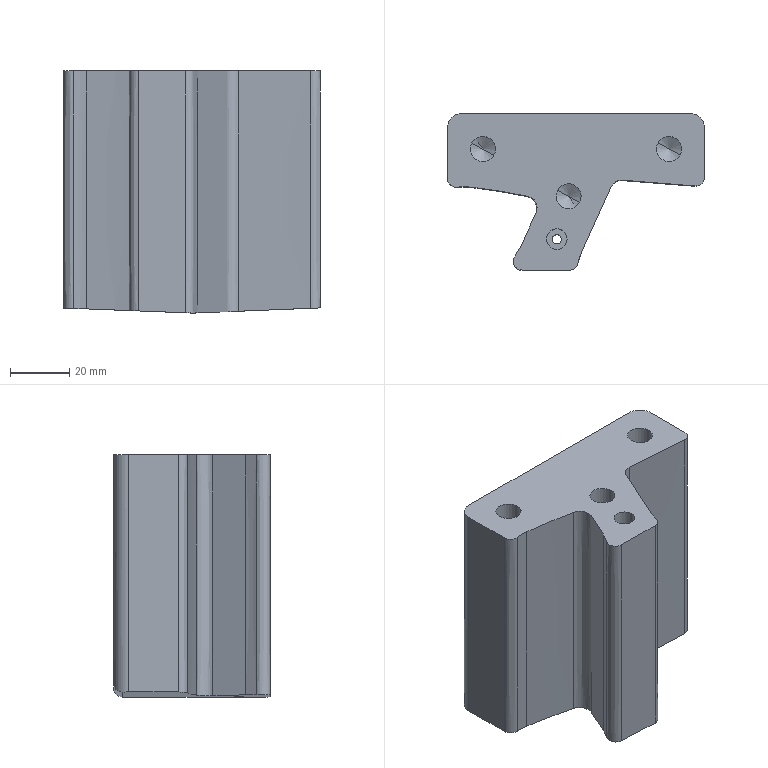Part | CATIA | 1 solid | 41 faces | box 87 x 53 x 82 mm | volume 218758 mm3 | cylinder 14 | other 12 | plane 9 | cone 6 | commonest cylinder face diameters 8.5 x6 3.2 x2 6 x2 7 x2 10 x2
STEP:
#1=CARTESIAN_POINT('',(-84.,32.5,41.546));
#2=VERTEX_POINT('',#1);
#3=CARTESIAN_POINT('',(-87.73,34.538,44.));
#4=VERTEX_POINT('',#3);
#5=CARTESIAN_POINT('',(-85.865,33.519,42.773));
#6=DIRECTION('',(-0.76,0.4152,0.5));
#7=VECTOR('',#6,1.);
#8=LINE('',#5,#7);
#9=EDGE_CURVE('',#2,#4,#8,.T.);
#10=ORIENTED_EDGE('',*,*,#9,.T.);
#11=CARTESIAN_POINT('',(-80.27,30.462,44.));
#12=VERTEX_POINT('',#11);
#13=CARTESIAN_POINT('',(-84.,32.5,44.));
#14=DIRECTION('',(0.,0.,1.));
#15=AXIS2_PLACEMENT_3D('',#13,#14,$);
#16=CIRCLE('',#15,4.25);
#17=EDGE_CURVE('',#12,#4,#16,.F.);
#18=ORIENTED_EDGE('',*,*,#17,.F.);
#19=CARTESIAN_POINT('',(-82.135,31.481,42.773));
#20=DIRECTION('',(0.76,-0.4152,0.5));
#21=VECTOR('',#20,1.);
#22=LINE('',#19,#21);
#23=EDGE_CURVE('',#2,#12,#22,.T.);
#24=ORIENTED_EDGE('',*,*,#23,.F.);
#25=EDGE_LOOP('',(#10,#18,#24));
#26=FACE_OUTER_BOUND('',#25,.T.);
#27=CARTESIAN_POINT('',(-84.,32.5,41.546));
#28=DIRECTION('',(0.,0.,1.));
#29=DIRECTION('',(0.8776,-0.4794,0.));
#30=AXIS2_PLACEMENT_3D('',#27,#28,#29);
#31=CONICAL_SURFACE('',#30,0.,1.047);
#32=ADVANCED_FACE('',(#26),#31,.F.);
#33=ORIENTED_EDGE('',*,*,#23,.T.);
#34=CARTESIAN_POINT('',(-84.,32.5,44.));
#35=DIRECTION('',(0.,0.,1.));
#36=AXIS2_PLACEMENT_3D('',#34,#35,$);
#37=CIRCLE('',#36,4.25);
#38=EDGE_CURVE('',#4,#12,#37,.F.);
#39=ORIENTED_EDGE('',*,*,#38,.F.);
#40=ORIENTED_EDGE('',*,*,#9,.F.);
#41=EDGE_LOOP('',(#33,#39,#40));
#42=FACE_OUTER_BOUND('',#41,.T.);
#43=ADVANCED_FACE('',(#42),#31,.F.);
#44=CARTESIAN_POINT('',(-87.73,34.538,69.));
#45=VERTEX_POINT('',#44);
#46=CARTESIAN_POINT('',(-80.27,30.462,69.));
#47=VERTEX_POINT('',#46);
#48=CARTESIAN_POINT('',(-84.,32.5,69.));
#49=DIRECTION('',(0.,0.,-1.));
#50=AXIS2_PLACEMENT_3D('',#48,#49,$);
#51=CIRCLE('',#50,4.25);
#52=EDGE_CURVE('',#45,#47,#51,.F.);
#53=ORIENTED_EDGE('',*,*,#52,.T.);
#54=CARTESIAN_POINT('',(-80.27,30.462,56.655));
#55=DIRECTION('',(0.,0.,-1.));
#56=VECTOR('',#55,1.);
#57=LINE('',#54,#56);
#58=EDGE_CURVE('',#12,#47,#57,.F.);
#59=ORIENTED_EDGE('',*,*,#58,.F.);
#60=ORIENTED_EDGE('',*,*,#17,.T.);
#61=CARTESIAN_POINT('',(-87.73,34.538,56.655));
#62=DIRECTION('',(0.,0.,-1.));
#63=VECTOR('',#62,1.);
#64=LINE('',#61,#63);
#65=EDGE_CURVE('',#4,#45,#64,.F.);
#66=ORIENTED_EDGE('',*,*,#65,.T.);
#67=EDGE_LOOP('',(#53,#59,#60,#66));
#68=FACE_OUTER_BOUND('',#67,.T.);
#69=CARTESIAN_POINT('',(-84.,32.5,68.9));
#70=DIRECTION('',(0.,0.,-1.));
#71=DIRECTION('',(0.8776,-0.4794,0.));
#72=AXIS2_PLACEMENT_3D('',#69,#70,#71);
#73=CYLINDRICAL_SURFACE('',#72,4.25);
#74=ADVANCED_FACE('',(#68),#73,.F.);
#75=CARTESIAN_POINT('',(-84.,32.5,69.));
#76=DIRECTION('',(0.,0.,-1.));
#77=AXIS2_PLACEMENT_3D('',#75,#76,$);
#78=CIRCLE('',#77,4.25);
#79=EDGE_CURVE('',#47,#45,#78,.F.);
#80=ORIENTED_EDGE('',*,*,#79,.T.);
#81=ORIENTED_EDGE('',*,*,#65,.F.);
#82=ORIENTED_EDGE('',*,*,#38,.T.);
#83=ORIENTED_EDGE('',*,*,#58,.T.);
#84=EDGE_LOOP('',(#80,#81,#82,#83));
#85=FACE_OUTER_BOUND('',#84,.T.);
#86=ADVANCED_FACE('',(#85),#73,.F.);
#87=CARTESIAN_POINT('',(-50.,48.5,41.546));
#88=VERTEX_POINT('',#87);
#89=CARTESIAN_POINT('',(-53.73,50.538,44.));
#90=VERTEX_POINT('',#89);
#91=CARTESIAN_POINT('',(-51.865,49.519,42.773));
#92=DIRECTION('',(-0.76,0.4152,0.5));
#93=VECTOR('',#92,1.);
#94=LINE('',#91,#93);
#95=EDGE_CURVE('',#88,#90,#94,.T.);
#96=ORIENTED_EDGE('',*,*,#95,.T.);
#97=CARTESIAN_POINT('',(-46.27,46.462,44.));
#98=VERTEX_POINT('',#97);
#99=CARTESIAN_POINT('',(-50.,48.5,44.));
#100=DIRECTION('',(0.,0.,1.));
#101=AXIS2_PLACEMENT_3D('',#99,#100,$);
#102=CIRCLE('',#101,4.25);
#103=EDGE_CURVE('',#98,#90,#102,.F.);
#104=ORIENTED_EDGE('',*,*,#103,.F.);
#105=CARTESIAN_POINT('',(-48.135,47.481,42.773));
#106=DIRECTION('',(0.76,-0.4152,0.5));
#107=VECTOR('',#106,1.);
#108=LINE('',#105,#107);
#109=EDGE_CURVE('',#88,#98,#108,.T.);
#110=ORIENTED_EDGE('',*,*,#109,.F.);
#111=EDGE_LOOP('',(#96,#104,#110));
#112=FACE_OUTER_BOUND('',#111,.T.);
#113=CARTESIAN_POINT('',(-50.,48.5,41.546));
#114=DIRECTION('',(0.,0.,1.));
#115=DIRECTION('',(0.8776,-0.4794,0.));
#116=AXIS2_PLACEMENT_3D('',#113,#114,#115);
#117=CONICAL_SURFACE('',#116,0.,1.047);
#118=ADVANCED_FACE('',(#112),#117,.F.);
#119=ORIENTED_EDGE('',*,*,#109,.T.);
#120=CARTESIAN_POINT('',(-50.,48.5,44.));
#121=DIRECTION('',(0.,0.,1.));
#122=AXIS2_PLACEMENT_3D('',#120,#121,$);
#123=CIRCLE('',#122,4.25);
#124=EDGE_CURVE('',#90,#98,#123,.F.);
#125=ORIENTED_EDGE('',*,*,#124,.F.);
#126=ORIENTED_EDGE('',*,*,#95,.F.);
#127=EDGE_LOOP('',(#119,#125,#126));
#128=FACE_OUTER_BOUND('',#127,.T.);
#129=ADVANCED_FACE('',(#128),#117,.F.);
#130=CARTESIAN_POINT('',(-53.73,50.538,69.));
#131=VERTEX_POINT('',#130);
#132=CARTESIAN_POINT('',(-46.27,46.462,69.));
#133=VERTEX_POINT('',#132);
#134=CARTESIAN_POINT('',(-50.,48.5,69.));
#135=DIRECTION('',(0.,0.,-1.));
#136=AXIS2_PLACEMENT_3D('',#134,#135,$);
#137=CIRCLE('',#136,4.25);
#138=EDGE_CURVE('',#131,#133,#137,.F.);
#139=ORIENTED_EDGE('',*,*,#138,.T.);
#140=CARTESIAN_POINT('',(-46.27,46.462,56.655));
#141=DIRECTION('',(0.,0.,-1.));
#142=VECTOR('',#141,1.);
#143=LINE('',#140,#142);
#144=EDGE_CURVE('',#98,#133,#143,.F.);
#145=ORIENTED_EDGE('',*,*,#144,.F.);
#146=ORIENTED_EDGE('',*,*,#103,.T.);
#147=CARTESIAN_POINT('',(-53.73,50.538,56.655));
#148=DIRECTION('',(0.,0.,-1.));
#149=VECTOR('',#148,1.);
#150=LINE('',#147,#149);
#151=EDGE_CURVE('',#90,#131,#150,.F.);
#152=ORIENTED_EDGE('',*,*,#151,.T.);
#153=EDGE_LOOP('',(#139,#145,#146,#152));
#154=FACE_OUTER_BOUND('',#153,.T.);
#155=CARTESIAN_POINT('',(-50.,48.5,68.9));
#156=DIRECTION('',(0.,0.,-1.));
#157=DIRECTION('',(0.8776,-0.4794,0.));
#158=AXIS2_PLACEMENT_3D('',#155,#156,#157);
#159=CYLINDRICAL_SURFACE('',#158,4.25);
#160=ADVANCED_FACE('',(#154),#159,.F.);
#161=CARTESIAN_POINT('',(-50.,48.5,69.));
#162=DIRECTION('',(0.,0.,-1.));
#163=AXIS2_PLACEMENT_3D('',#161,#162,$);
#164=CIRCLE('',#163,4.25);
#165=EDGE_CURVE('',#133,#131,#164,.F.);
#166=ORIENTED_EDGE('',*,*,#165,.T.);
#167=ORIENTED_EDGE('',*,*,#151,.F.);
#168=ORIENTED_EDGE('',*,*,#124,.T.);
#169=ORIENTED_EDGE('',*,*,#144,.T.);
#170=EDGE_LOOP('',(#166,#167,#168,#169));
#171=FACE_OUTER_BOUND('',#170,.T.);
#172=ADVANCED_FACE('',(#171),#159,.F.);
#173=CARTESIAN_POINT('',(-113.,48.5,41.546));
#174=VERTEX_POINT('',#173);
#175=CARTESIAN_POINT('',(-116.73,50.538,44.));
#176=VERTEX_POINT('',#175);
#177=CARTESIAN_POINT('',(-114.865,49.519,42.773));
#178=DIRECTION('',(-0.76,0.4152,0.5));
#179=VECTOR('',#178,1.);
#180=LINE('',#177,#179);
#181=EDGE_CURVE('',#174,#176,#180,.T.);
#182=ORIENTED_EDGE('',*,*,#181,.T.);
#183=CARTESIAN_POINT('',(-109.27,46.462,44.));
#184=VERTEX_POINT('',#183);
#185=CARTESIAN_POINT('',(-113.,48.5,44.));
#186=DIRECTION('',(0.,0.,1.));
#187=AXIS2_PLACEMENT_3D('',#185,#186,$);
#188=CIRCLE('',#187,4.25);
#189=EDGE_CURVE('',#184,#176,#188,.F.);
#190=ORIENTED_EDGE('',*,*,#189,.F.);
#191=CARTESIAN_POINT('',(-111.135,47.481,42.773));
#192=DIRECTION('',(0.76,-0.4152,0.5));
#193=VECTOR('',#192,1.);
#194=LINE('',#191,#193);
#195=EDGE_CURVE('',#174,#184,#194,.T.);
#196=ORIENTED_EDGE('',*,*,#195,.F.);
#197=EDGE_LOOP('',(#182,#190,#196));
#198=FACE_OUTER_BOUND('',#197,.T.);
#199=CARTESIAN_POINT('',(-113.,48.5,41.546));
#200=DIRECTION('',(0.,0.,1.));
#201=DIRECTION('',(0.8776,-0.4794,0.));
#202=AXIS2_PLACEMENT_3D('',#199,#200,#201);
#203=CONICAL_SURFACE('',#202,0.,1.047);
#204=ADVANCED_FACE('',(#198),#203,.F.);
#205=ORIENTED_EDGE('',*,*,#195,.T.);
#206=CARTESIAN_POINT('',(-113.,48.5,44.));
#207=DIRECTION('',(0.,0.,1.));
#208=AXIS2_PLACEMENT_3D('',#206,#207,$);
#209=CIRCLE('',#208,4.25);
#210=EDGE_CURVE('',#176,#184,#209,.F.);
#211=ORIENTED_EDGE('',*,*,#210,.F.);
#212=ORIENTED_EDGE('',*,*,#181,.F.);
#213=EDGE_LOOP('',(#205,#211,#212));
#214=FACE_OUTER_BOUND('',#213,.T.);
#215=ADVANCED_FACE('',(#214),#203,.F.);
#216=CARTESIAN_POINT('',(-116.73,50.538,69.));
#217=VERTEX_POINT('',#216);
#218=CARTESIAN_POINT('',(-109.27,46.462,69.));
#219=VERTEX_POINT('',#218);
#220=CARTESIAN_POINT('',(-113.,48.5,69.));
#221=DIRECTION('',(0.,0.,-1.));
#222=AXIS2_PLACEMENT_3D('',#220,#221,$);
#223=CIRCLE('',#222,4.25);
#224=EDGE_CURVE('',#217,#219,#223,.F.);
#225=ORIENTED_EDGE('',*,*,#224,.T.);
#226=CARTESIAN_POINT('',(-109.27,46.462,56.655));
#227=DIRECTION('',(0.,0.,-1.));
#228=VECTOR('',#227,1.);
#229=LINE('',#226,#228);
#230=EDGE_CURVE('',#184,#219,#229,.F.);
#231=ORIENTED_EDGE('',*,*,#230,.F.);
#232=ORIENTED_EDGE('',*,*,#189,.T.);
#233=CARTESIAN_POINT('',(-116.73,50.538,56.655));
#234=DIRECTION('',(0.,0.,-1.));
#235=VECTOR('',#234,1.);
#236=LINE('',#233,#235);
#237=EDGE_CURVE('',#176,#217,#236,.F.);
#238=ORIENTED_EDGE('',*,*,#237,.T.);
#239=EDGE_LOOP('',(#225,#231,#232,#238));
#240=FACE_OUTER_BOUND('',#239,.T.);
#241=CARTESIAN_POINT('',(-113.,48.5,68.9));
#242=DIRECTION('',(0.,0.,-1.));
#243=DIRECTION('',(0.8776,-0.4794,0.));
#244=AXIS2_PLACEMENT_3D('',#241,#242,#243);
#245=CYLINDRICAL_SURFACE('',#244,4.25);
#246=ADVANCED_FACE('',(#240),#245,.F.);
#247=CARTESIAN_POINT('',(-113.,48.5,69.));
#248=DIRECTION('',(0.,0.,-1.));
#249=AXIS2_PLACEMENT_3D('',#247,#248,$);
#250=CIRCLE('',#249,4.25);
#251=EDGE_CURVE('',#219,#217,#250,.F.);
#252=ORIENTED_EDGE('',*,*,#251,.T.);
#253=ORIENTED_EDGE('',*,*,#237,.F.);
#254=ORIENTED_EDGE('',*,*,#210,.T.);
#255=ORIENTED_EDGE('',*,*,#230,.T.);
#256=EDGE_LOOP('',(#252,#253,#254,#255));
#257=FACE_OUTER_BOUND('',#256,.T.);
#258=ADVANCED_FACE('',(#257),#245,.F.);
#259=CARTESIAN_POINT('',(-38.,55.5,-11.244));
#260=VERTEX_POINT('',#259);
#261=CARTESIAN_POINT('',(-38.,38.985,-11.244));
#262=VERTEX_POINT('',#261);
#263=CARTESIAN_POINT('',(-38.,47.243,-11.244));
#264=DIRECTION('',(0.,-1.,0.));
#265=VECTOR('',#264,1.);
#266=LINE('',#263,#265);
#267=EDGE_CURVE('',#260,#262,#266,.T.);
#268=ORIENTED_EDGE('',*,*,#267,.F.);
#269=CARTESIAN_POINT('',(-38.,55.5,69.));
#270=VERTEX_POINT('',#269);
#271=CARTESIAN_POINT('',(-38.,55.5,28.878));
#272=DIRECTION('',(0.,0.,1.));
#273=VECTOR('',#272,1.);
#274=LINE('',#271,#273);
#275=EDGE_CURVE('',#260,#270,#274,.T.);
#276=ORIENTED_EDGE('',*,*,#275,.T.);
#277=CARTESIAN_POINT('',(-38.,38.985,69.));
#278=VERTEX_POINT('',#277);
#279=CARTESIAN_POINT('',(-38.,47.243,69.));
#280=DIRECTION('',(0.,-1.,0.));
#281=VECTOR('',#280,1.);
#282=LINE('',#279,#281);
#283=EDGE_CURVE('',#270,#278,#282,.T.);
#284=ORIENTED_EDGE('',*,*,#283,.T.);
#285=CARTESIAN_POINT('',(-38.,38.985,28.878));
#286=DIRECTION('',(0.,0.,1.));
#287=VECTOR('',#286,1.);
#288=LINE('',#285,#287);
#289=EDGE_CURVE('',#262,#278,#288,.T.);
#290=ORIENTED_EDGE('',*,*,#289,.F.);
#291=EDGE_LOOP('',(#268,#276,#284,#290));
#292=FACE_OUTER_BOUND('',#291,.T.);
#293=CARTESIAN_POINT('',(-38.,55.5,0.));
#294=DIRECTION('',(-1.,0.,0.));
#295=DIRECTION('',(0.,-1.,0.));
#296=AXIS2_PLACEMENT_3D('',#293,#294,#295);
#297=PLANE('',#296);
#298=ADVANCED_FACE('',(#292),#297,.F.);
#299=CARTESIAN_POINT('',(-125.,38.571,-11.275));
#300=VERTEX_POINT('',#299);
#301=CARTESIAN_POINT('',(-125.,55.5,-11.275));
#302=VERTEX_POINT('',#301);
#303=CARTESIAN_POINT('',(-125.,47.035,-11.275));
#304=DIRECTION('',(0.,1.,0.));
#305=VECTOR('',#304,1.);
#306=LINE('',#303,#305);
#307=EDGE_CURVE('',#300,#302,#306,.T.);
#308=ORIENTED_EDGE('',*,*,#307,.F.);
#309=CARTESIAN_POINT('',(-125.,38.571,69.));
#310=VERTEX_POINT('',#309);
#311=CARTESIAN_POINT('',(-125.,38.571,28.862));
#312=DIRECTION('',(0.,0.,1.));
#313=VECTOR('',#312,1.);
#314=LINE('',#311,#313);
#315=EDGE_CURVE('',#300,#310,#314,.T.);
#316=ORIENTED_EDGE('',*,*,#315,.T.);
#317=CARTESIAN_POINT('',(-125.,55.5,69.));
#318=VERTEX_POINT('',#317);
#319=CARTESIAN_POINT('',(-125.,47.035,69.));
#320=DIRECTION('',(0.,1.,0.));
#321=VECTOR('',#320,1.);
#322=LINE('',#319,#321);
#323=EDGE_CURVE('',#310,#318,#322,.T.);
#324=ORIENTED_EDGE('',*,*,#323,.T.);
#325=CARTESIAN_POINT('',(-125.,55.5,28.862));
#326=DIRECTION('',(0.,0.,1.));
#327=VECTOR('',#326,1.);
#328=LINE('',#325,#327);
#329=EDGE_CURVE('',#302,#318,#328,.T.);
#330=ORIENTED_EDGE('',*,*,#329,.F.);
#331=EDGE_LOOP('',(#308,#316,#324,#330));
#332=FACE_OUTER_BOUND('',#331,.T.);
#333=CARTESIAN_POINT('',(-125.,38.571,0.));
#334=DIRECTION('',(1.,0.,0.));
#335=DIRECTION('',(0.,1.,0.));
#336=AXIS2_PLACEMENT_3D('',#333,#334,#335);
#337=PLANE('',#336);
#338=ADVANCED_FACE('',(#332),#337,.F.);
#339=CARTESIAN_POINT('',(-121.659,35.59,-11.407));
#340=VERTEX_POINT('',#339);
#341=CARTESIAN_POINT('',(-125.,38.571,-11.275));
#342=CARTESIAN_POINT('',(-125.,37.559,-11.275));
#343=CARTESIAN_POINT('',(-124.575,36.547,-11.292));
#344=CARTESIAN_POINT('',(-123.717,35.781,-11.326));
#345=CARTESIAN_POINT('',(-122.662,35.475,-11.367));
#346=CARTESIAN_POINT('',(-121.659,35.59,-11.407));
#347=B_SPLINE_CURVE_WITH_KNOTS('',5,(#341,#342,#343,#344,#345,#346),.UNSPECIFIED.,.F.,.U.,(6,6),(0.,7.151),.UNSPECIFIED.);
#348=EDGE_CURVE('',#300,#340,#347,.T.);
#349=ORIENTED_EDGE('',*,*,#348,.T.);
#350=CARTESIAN_POINT('',(-121.659,35.59,69.));
#351=VERTEX_POINT('',#350);
#352=CARTESIAN_POINT('',(-121.659,35.59,28.61));
#353=DIRECTION('',(0.,0.,1.));
#354=VECTOR('',#353,1.);
#355=LINE('',#352,#354);
#356=EDGE_CURVE('',#340,#351,#355,.T.);
#357=ORIENTED_EDGE('',*,*,#356,.T.);
#358=CARTESIAN_POINT('',(-121.659,35.59,69.));
#359=CARTESIAN_POINT('',(-122.663,35.475,69.));
#360=CARTESIAN_POINT('',(-123.717,35.781,69.));
#361=CARTESIAN_POINT('',(-124.576,36.547,69.));
#362=CARTESIAN_POINT('',(-125.,37.56,69.));
#363=CARTESIAN_POINT('',(-125.,38.571,69.));
#364=B_SPLINE_CURVE_WITH_KNOTS('',5,(#358,#359,#360,#361,#362,#363),.UNSPECIFIED.,.F.,.U.,(6,6),(0.,7.148),.UNSPECIFIED.);
#365=EDGE_CURVE('',#351,#310,#364,.T.);
#366=ORIENTED_EDGE('',*,*,#365,.T.);
#367=ORIENTED_EDGE('',*,*,#315,.F.);
#368=EDGE_LOOP('',(#349,#357,#366,#367));
#369=FACE_OUTER_BOUND('',#368,.T.);
#370=CARTESIAN_POINT('',(-121.659,35.59,0.));
#371=CARTESIAN_POINT('',(-122.663,35.475,0.));
#372=CARTESIAN_POINT('',(-123.717,35.781,0.));
#373=CARTESIAN_POINT('',(-124.576,36.547,0.));
#374=CARTESIAN_POINT('',(-125.,37.56,0.));
#375=CARTESIAN_POINT('',(-125.,38.571,0.));
#376=B_SPLINE_CURVE_WITH_KNOTS('',5,(#370,#371,#372,#373,#374,#375),.UNSPECIFIED.,.F.,.U.,(6,6),(5.675,10.828),.UNSPECIFIED.);
#377=DIRECTION('',(0.,0.,1.));
#378=VECTOR('',#377,1.);
#379=SURFACE_OF_LINEAR_EXTRUSION('',#376,#378);
#380=ADVANCED_FACE('',(#369),#379,.F.);
#381=CARTESIAN_POINT('',(-117.084,35.588,-11.587));
#382=VERTEX_POINT('',#381);
#383=CARTESIAN_POINT('',(-117.084,35.588,-11.587));
#384=CARTESIAN_POINT('',(-118.601,35.763,-11.527));
#385=CARTESIAN_POINT('',(-120.142,35.764,-11.466));
#386=CARTESIAN_POINT('',(-121.659,35.59,-11.407));
#387=B_SPLINE_CURVE_WITH_KNOTS('',3,(#383,#384,#385,#386),.UNSPECIFIED.,.F.,.U.,(4,4),(0.,6.481),.UNSPECIFIED.);
#388=EDGE_CURVE('',#382,#340,#387,.T.);
#389=ORIENTED_EDGE('',*,*,#388,.F.);
#390=CARTESIAN_POINT('',(-117.084,35.588,69.));
#391=VERTEX_POINT('',#390);
#392=CARTESIAN_POINT('',(-117.084,35.588,28.61));
#393=DIRECTION('',(0.,0.,1.));
#394=VECTOR('',#393,1.);
#395=LINE('',#392,#394);
#396=EDGE_CURVE('',#382,#391,#395,.T.);
#397=ORIENTED_EDGE('',*,*,#396,.T.);
#398=CARTESIAN_POINT('',(-117.084,35.588,69.));
#399=CARTESIAN_POINT('',(-118.601,35.763,69.));
#400=CARTESIAN_POINT('',(-120.142,35.764,69.));
#401=CARTESIAN_POINT('',(-121.659,35.59,69.));
#402=B_SPLINE_CURVE_WITH_KNOTS('',3,(#398,#399,#400,#401),.UNSPECIFIED.,.F.,.U.,(4,4),(0.,6.476),.UNSPECIFIED.);
#403=EDGE_CURVE('',#391,#351,#402,.T.);
#404=ORIENTED_EDGE('',*,*,#403,.T.);
#405=ORIENTED_EDGE('',*,*,#356,.F.);
#406=EDGE_LOOP('',(#389,#397,#404,#405));
#407=FACE_OUTER_BOUND('',#406,.T.);
#408=CARTESIAN_POINT('',(-117.084,35.588,0.));
#409=CARTESIAN_POINT('',(-118.602,35.763,0.));
#410=CARTESIAN_POINT('',(-120.14,35.764,0.));
#411=CARTESIAN_POINT('',(-121.659,35.59,0.));
#412=B_SPLINE_CURVE_WITH_KNOTS('',3,(#408,#409,#410,#411),.UNSPECIFIED.,.F.,.U.,(4,4),(3.211,7.799),.UNSPECIFIED.);
#413=DIRECTION('',(0.,0.,1.));
#414=VECTOR('',#413,1.);
#415=SURFACE_OF_LINEAR_EXTRUSION('',#412,#414);
#416=ADVANCED_FACE('',(#407),#415,.F.);
#417=CARTESIAN_POINT('',(-97.856,32.48,-12.343));
#418=VERTEX_POINT('',#417);
#419=CARTESIAN_POINT('',(-97.856,32.48,-12.343));
#420=CARTESIAN_POINT('',(-104.214,33.804,-12.093));
#421=CARTESIAN_POINT('',(-110.634,34.842,-11.84));
#422=CARTESIAN_POINT('',(-117.084,35.588,-11.587));
#423=B_SPLINE_CURVE_WITH_KNOTS('',3,(#419,#420,#421,#422),.UNSPECIFIED.,.F.,.U.,(4,4),(0.,27.571),.UNSPECIFIED.);
#424=EDGE_CURVE('',#418,#382,#423,.T.);
#425=ORIENTED_EDGE('',*,*,#424,.F.);
#426=CARTESIAN_POINT('',(-97.856,32.48,69.));
#427=VERTEX_POINT('',#426);
#428=CARTESIAN_POINT('',(-97.856,32.48,28.61));
#429=DIRECTION('',(0.,0.,1.));
#430=VECTOR('',#429,1.);
#431=LINE('',#428,#430);
#432=EDGE_CURVE('',#418,#427,#431,.T.);
#433=ORIENTED_EDGE('',*,*,#432,.T.);
#434=CARTESIAN_POINT('',(-97.856,32.48,69.));
#435=CARTESIAN_POINT('',(-104.213,33.804,69.));
#436=CARTESIAN_POINT('',(-110.634,34.842,69.));
#437=CARTESIAN_POINT('',(-117.084,35.588,69.));
#438=B_SPLINE_CURVE_WITH_KNOTS('',3,(#434,#435,#436,#437),.UNSPECIFIED.,.F.,.U.,(4,4),(0.,27.55),.UNSPECIFIED.);
#439=EDGE_CURVE('',#427,#391,#438,.T.);
#440=ORIENTED_EDGE('',*,*,#439,.T.);
#441=ORIENTED_EDGE('',*,*,#396,.F.);
#442=EDGE_LOOP('',(#425,#433,#440,#441));
#443=FACE_OUTER_BOUND('',#442,.T.);
#444=CARTESIAN_POINT('',(-97.856,32.48,0.));
#445=CARTESIAN_POINT('',(-104.215,33.804,0.));
#446=CARTESIAN_POINT('',(-110.633,34.841,0.));
#447=CARTESIAN_POINT('',(-117.084,35.588,0.));
#448=B_SPLINE_CURVE_WITH_KNOTS('',3,(#444,#445,#446,#447),.UNSPECIFIED.,.F.,.U.,(4,4),(13.641,33.127),.UNSPECIFIED.);
#449=DIRECTION('',(0.,0.,1.));
#450=VECTOR('',#449,1.);
#451=SURFACE_OF_LINEAR_EXTRUSION('',#448,#450);
#452=ADVANCED_FACE('',(#443),#451,.F.);
#453=CARTESIAN_POINT('',(-95.029,26.911,-12.454));
#454=VERTEX_POINT('',#453);
#455=CARTESIAN_POINT('',(-95.029,26.911,-12.454));
#456=CARTESIAN_POINT('',(-94.437,28.216,-12.477));
#457=CARTESIAN_POINT('',(-94.425,29.789,-12.478));
#458=CARTESIAN_POINT('',(-95.178,31.271,-12.448));
#459=CARTESIAN_POINT('',(-96.454,32.188,-12.398));
#460=CARTESIAN_POINT('',(-97.856,32.48,-12.343));
#461=B_SPLINE_CURVE_WITH_KNOTS('',5,(#455,#456,#457,#458,#459,#460),.UNSPECIFIED.,.F.,.U.,(6,6),(0.,10.137),.UNSPECIFIED.);
#462=EDGE_CURVE('',#454,#418,#461,.T.);
#463=ORIENTED_EDGE('',*,*,#462,.F.);
#464=CARTESIAN_POINT('',(-95.029,26.911,69.));
#465=VERTEX_POINT('',#464);
#466=CARTESIAN_POINT('',(-95.029,26.911,28.61));
#467=DIRECTION('',(0.,0.,1.));
#468=VECTOR('',#467,1.);
#469=LINE('',#466,#468);
#470=EDGE_CURVE('',#454,#465,#469,.T.);
#471=ORIENTED_EDGE('',*,*,#470,.T.);
#472=CARTESIAN_POINT('',(-95.029,26.911,69.));
#473=CARTESIAN_POINT('',(-94.437,28.216,69.));
#474=CARTESIAN_POINT('',(-94.426,29.788,69.));
#475=CARTESIAN_POINT('',(-95.176,31.27,69.));
#476=CARTESIAN_POINT('',(-96.453,32.188,69.));
#477=CARTESIAN_POINT('',(-97.856,32.48,69.));
#478=B_SPLINE_CURVE_WITH_KNOTS('',5,(#472,#473,#474,#475,#476,#477),.UNSPECIFIED.,.F.,.U.,(6,6),(0.,10.134),.UNSPECIFIED.);
#479=EDGE_CURVE('',#465,#427,#478,.T.);
#480=ORIENTED_EDGE('',*,*,#479,.T.);
#481=ORIENTED_EDGE('',*,*,#432,.F.);
#482=EDGE_LOOP('',(#463,#471,#480,#481));
#483=FACE_OUTER_BOUND('',#482,.T.);
#484=CARTESIAN_POINT('',(-95.029,26.911,0.));
#485=CARTESIAN_POINT('',(-94.437,28.216,0.));
#486=CARTESIAN_POINT('',(-94.425,29.788,0.));
#487=CARTESIAN_POINT('',(-95.177,31.27,0.));
#488=CARTESIAN_POINT('',(-96.453,32.188,0.));
#489=CARTESIAN_POINT('',(-97.856,32.48,0.));
#490=B_SPLINE_CURVE_WITH_KNOTS('',5,(#484,#485,#486,#487,#488,#489),.UNSPECIFIED.,.F.,.U.,(6,6),(5.259,12.771),.UNSPECIFIED.);
#491=DIRECTION('',(0.,0.,1.));
#492=VECTOR('',#491,1.);
#493=SURFACE_OF_LINEAR_EXTRUSION('',#490,#492);
#494=ADVANCED_FACE('',(#483),#493,.F.);
#495=CARTESIAN_POINT('',(-100.034,15.873,-12.257));
#496=VERTEX_POINT('',#495);
#497=CARTESIAN_POINT('',(-100.034,15.873,-12.257));
#498=CARTESIAN_POINT('',(-98.367,19.553,-12.323));
#499=CARTESIAN_POINT('',(-96.699,23.232,-12.388));
#500=CARTESIAN_POINT('',(-95.029,26.911,-12.454));
#501=B_SPLINE_CURVE_WITH_KNOTS('',3,(#497,#498,#499,#500),.UNSPECIFIED.,.F.,.U.,(4,4),(0.,17.142),.UNSPECIFIED.);
#502=EDGE_CURVE('',#496,#454,#501,.T.);
#503=ORIENTED_EDGE('',*,*,#502,.F.);
#504=CARTESIAN_POINT('',(-100.034,15.873,69.));
#505=VERTEX_POINT('',#504);
#506=CARTESIAN_POINT('',(-100.034,15.873,28.61));
#507=DIRECTION('',(0.,0.,1.));
#508=VECTOR('',#507,1.);
#509=LINE('',#506,#508);
#510=EDGE_CURVE('',#496,#505,#509,.T.);
#511=ORIENTED_EDGE('',*,*,#510,.T.);
#512=CARTESIAN_POINT('',(-100.034,15.873,69.));
#513=CARTESIAN_POINT('',(-98.367,19.553,69.));
#514=CARTESIAN_POINT('',(-96.699,23.232,69.));
#515=CARTESIAN_POINT('',(-95.029,26.911,69.));
#516=B_SPLINE_CURVE_WITH_KNOTS('',3,(#512,#513,#514,#515),.UNSPECIFIED.,.F.,.U.,(4,4),(0.,17.14),.UNSPECIFIED.);
#517=EDGE_CURVE('',#505,#465,#516,.T.);
#518=ORIENTED_EDGE('',*,*,#517,.T.);
#519=ORIENTED_EDGE('',*,*,#470,.F.);
#520=EDGE_LOOP('',(#503,#511,#518,#519));
#521=FACE_OUTER_BOUND('',#520,.T.);
#522=CARTESIAN_POINT('',(-100.034,15.873,0.));
#523=CARTESIAN_POINT('',(-98.367,19.553,0.));
#524=CARTESIAN_POINT('',(-96.699,23.232,0.));
#525=CARTESIAN_POINT('',(-95.029,26.911,0.));
#526=B_SPLINE_CURVE_WITH_KNOTS('',3,(#522,#523,#524,#525),.UNSPECIFIED.,.F.,.U.,(4,4),(8.484,20.604),.UNSPECIFIED.);
#527=DIRECTION('',(0.,0.,1.));
#528=VECTOR('',#527,1.);
#529=SURFACE_OF_LINEAR_EXTRUSION('',#526,#528);
#530=ADVANCED_FACE('',(#521),#529,.F.);
#531=CARTESIAN_POINT('',(-102.138,12.277,-12.174));
#532=VERTEX_POINT('',#531);
#533=CARTESIAN_POINT('',(-100.034,15.873,-12.257));
#534=CARTESIAN_POINT('',(-100.607,14.606,-12.235));
#535=CARTESIAN_POINT('',(-101.315,13.397,-12.207));
#536=CARTESIAN_POINT('',(-102.138,12.277,-12.174));
#537=B_SPLINE_CURVE_WITH_KNOTS('',3,(#533,#534,#535,#536),.UNSPECIFIED.,.F.,.U.,(4,4),(0.,5.899),.UNSPECIFIED.);
#538=EDGE_CURVE('',#496,#532,#537,.T.);
#539=ORIENTED_EDGE('',*,*,#538,.T.);
#540=CARTESIAN_POINT('',(-102.138,12.277,69.));
#541=VERTEX_POINT('',#540);
#542=CARTESIAN_POINT('',(-102.138,12.277,28.61));
#543=DIRECTION('',(0.,0.,1.));
#544=VECTOR('',#543,1.);
#545=LINE('',#542,#544);
#546=EDGE_CURVE('',#532,#541,#545,.T.);
#547=ORIENTED_EDGE('',*,*,#546,.T.);
#548=CARTESIAN_POINT('',(-102.138,12.277,69.));
#549=CARTESIAN_POINT('',(-101.315,13.397,69.));
#550=CARTESIAN_POINT('',(-100.607,14.606,69.));
#551=CARTESIAN_POINT('',(-100.034,15.873,69.));
#552=B_SPLINE_CURVE_WITH_KNOTS('',3,(#548,#549,#550,#551),.UNSPECIFIED.,.F.,.U.,(4,4),(0.,5.898),.UNSPECIFIED.);
#553=EDGE_CURVE('',#541,#505,#552,.T.);
#554=ORIENTED_EDGE('',*,*,#553,.T.);
#555=ORIENTED_EDGE('',*,*,#510,.F.);
#556=EDGE_LOOP('',(#539,#547,#554,#555));
#557=FACE_OUTER_BOUND('',#556,.T.);
#558=CARTESIAN_POINT('',(-102.138,12.277,0.));
#559=CARTESIAN_POINT('',(-101.314,13.398,0.));
#560=CARTESIAN_POINT('',(-100.608,14.605,0.));
#561=CARTESIAN_POINT('',(-100.034,15.873,0.));
#562=B_SPLINE_CURVE_WITH_KNOTS('',3,(#558,#559,#560,#561),.UNSPECIFIED.,.F.,.U.,(4,4),(2.924,7.101),.UNSPECIFIED.);
#563=DIRECTION('',(0.,0.,1.));
#564=VECTOR('',#563,1.);
#565=SURFACE_OF_LINEAR_EXTRUSION('',#562,#564);
#566=ADVANCED_FACE('',(#557),#565,.F.);
#567=CARTESIAN_POINT('',(-99.721,7.5,-12.269));
#568=VERTEX_POINT('',#567);
#569=CARTESIAN_POINT('',(-102.138,12.277,-12.174));
#570=CARTESIAN_POINT('',(-102.922,11.211,-12.144));
#571=CARTESIAN_POINT('',(-103.128,9.711,-12.135));
#572=CARTESIAN_POINT('',(-102.374,8.222,-12.165));
#573=CARTESIAN_POINT('',(-101.043,7.5,-12.217));
#574=CARTESIAN_POINT('',(-99.721,7.5,-12.269));
#575=B_SPLINE_CURVE_WITH_KNOTS('',5,(#569,#570,#571,#572,#573,#574),.UNSPECIFIED.,.F.,.U.,(6,6),(0.,9.356),.UNSPECIFIED.);
#576=EDGE_CURVE('',#532,#568,#575,.T.);
#577=ORIENTED_EDGE('',*,*,#576,.T.);
#578=CARTESIAN_POINT('',(-99.721,7.5,69.));
#579=VERTEX_POINT('',#578);
#580=CARTESIAN_POINT('',(-99.721,7.5,28.61));
#581=DIRECTION('',(0.,0.,1.));
#582=VECTOR('',#581,1.);
#583=LINE('',#580,#582);
#584=EDGE_CURVE('',#568,#579,#583,.T.);
#585=ORIENTED_EDGE('',*,*,#584,.T.);
#586=CARTESIAN_POINT('',(-99.721,7.5,69.));
#587=CARTESIAN_POINT('',(-101.044,7.5,69.));
#588=CARTESIAN_POINT('',(-102.374,8.223,69.));
#589=CARTESIAN_POINT('',(-103.128,9.71,69.));
#590=CARTESIAN_POINT('',(-102.922,11.211,69.));
#591=CARTESIAN_POINT('',(-102.138,12.277,69.));
#592=B_SPLINE_CURVE_WITH_KNOTS('',5,(#586,#587,#588,#589,#590,#591),.UNSPECIFIED.,.F.,.U.,(6,6),(0.,9.353),.UNSPECIFIED.);
#593=EDGE_CURVE('',#579,#541,#592,.T.);
#594=ORIENTED_EDGE('',*,*,#593,.T.);
#595=ORIENTED_EDGE('',*,*,#546,.F.);
#596=EDGE_LOOP('',(#577,#585,#594,#595));
#597=FACE_OUTER_BOUND('',#596,.T.);
#598=CARTESIAN_POINT('',(-99.721,7.5,0.));
#599=CARTESIAN_POINT('',(-101.044,7.5,0.));
#600=CARTESIAN_POINT('',(-102.375,8.223,0.));
#601=CARTESIAN_POINT('',(-103.127,9.71,0.));
#602=CARTESIAN_POINT('',(-102.922,11.211,0.));
#603=CARTESIAN_POINT('',(-102.138,12.277,0.));
#604=B_SPLINE_CURVE_WITH_KNOTS('',5,(#598,#599,#600,#601,#602,#603),.UNSPECIFIED.,.F.,.U.,(6,6),(4.97,12.069),.UNSPECIFIED.);
#605=DIRECTION('',(0.,0.,1.));
#606=VECTOR('',#605,1.);
#607=SURFACE_OF_LINEAR_EXTRUSION('',#604,#606);
#608=ADVANCED_FACE('',(#597),#607,.F.);
#609=CARTESIAN_POINT('',(-83.802,7.5,-12.895));
#610=VERTEX_POINT('',#609);
#611=CARTESIAN_POINT('',(-91.762,7.5,-12.582));
#612=DIRECTION('',(-0.9992,-0.000000028,0.0393));
#613=VECTOR('',#612,1.);
#614=LINE('',#611,#613);
#615=EDGE_CURVE('',#610,#568,#614,.T.);
#616=ORIENTED_EDGE('',*,*,#615,.F.);
#617=CARTESIAN_POINT('',(-83.802,7.5,69.));
#618=VERTEX_POINT('',#617);
#619=CARTESIAN_POINT('',(-83.802,7.5,28.052));
#620=DIRECTION('',(0.,0.,1.));
#621=VECTOR('',#620,1.);
#622=LINE('',#619,#621);
#623=EDGE_CURVE('',#610,#618,#622,.T.);
#624=ORIENTED_EDGE('',*,*,#623,.T.);
#625=CARTESIAN_POINT('',(-91.762,7.5,69.));
#626=DIRECTION('',(-1.,-0.000000028,0.));
#627=VECTOR('',#626,1.);
#628=LINE('',#625,#627);
#629=EDGE_CURVE('',#618,#579,#628,.T.);
#630=ORIENTED_EDGE('',*,*,#629,.T.);
#631=ORIENTED_EDGE('',*,*,#584,.F.);
#632=EDGE_LOOP('',(#616,#624,#630,#631));
#633=FACE_OUTER_BOUND('',#632,.T.);
#634=CARTESIAN_POINT('',(-83.802,7.5,0.));
#635=DIRECTION('',(-0.000000028,1.,0.));
#636=DIRECTION('',(-1.,-0.000000028,0.));
#637=AXIS2_PLACEMENT_3D('',#634,#635,#636);
#638=PLANE('',#637);
#639=ADVANCED_FACE('',(#633),#638,.F.);
#640=CARTESIAN_POINT('',(-80.872,9.856,-12.989));
#641=VERTEX_POINT('',#640);
#642=CARTESIAN_POINT('',(-81.142,9.112,-13.));
#643=VERTEX_POINT('',#642);
#644=CARTESIAN_POINT('',(-80.872,9.856,-12.989));
#645=CARTESIAN_POINT('',(-80.929,9.598,-12.991));
#646=CARTESIAN_POINT('',(-81.02,9.347,-12.995));
#647=CARTESIAN_POINT('',(-81.142,9.112,-13.));
#648=B_SPLINE_CURVE_WITH_KNOTS('',3,(#644,#645,#646,#647),.UNSPECIFIED.,.F.,.U.,(4,4),(0.,1.121),.UNSPECIFIED.);
#649=EDGE_CURVE('',#641,#643,#648,.T.);
#650=ORIENTED_EDGE('',*,*,#649,.F.);
#651=CARTESIAN_POINT('',(-80.872,9.856,69.));
#652=VERTEX_POINT('',#651);
#653=CARTESIAN_POINT('',(-80.872,9.856,28.61));
#654=DIRECTION('',(0.,0.,1.));
#655=VECTOR('',#654,1.);
#656=LINE('',#653,#655);
#657=EDGE_CURVE('',#641,#652,#656,.T.);
#658=ORIENTED_EDGE('',*,*,#657,.T.);
#659=CARTESIAN_POINT('',(-80.872,9.856,69.));
#660=CARTESIAN_POINT('',(-81.046,9.063,69.));
#661=CARTESIAN_POINT('',(-81.49,8.328,69.));
#662=CARTESIAN_POINT('',(-82.173,7.776,69.));
#663=CARTESIAN_POINT('',(-82.99,7.5,69.));
#664=CARTESIAN_POINT('',(-83.802,7.5,69.));
#665=B_SPLINE_CURVE_WITH_KNOTS('',5,(#659,#660,#661,#662,#663,#664),.UNSPECIFIED.,.F.,.U.,(6,6),(0.,5.745),.UNSPECIFIED.);
#666=EDGE_CURVE('',#652,#618,#665,.T.);
#667=ORIENTED_EDGE('',*,*,#666,.T.);
#668=ORIENTED_EDGE('',*,*,#623,.F.);
#669=CARTESIAN_POINT('',(-81.142,9.112,-13.));
#670=CARTESIAN_POINT('',(-81.521,8.387,-12.985));
#671=CARTESIAN_POINT('',(-82.165,7.798,-12.96));
#672=CARTESIAN_POINT('',(-82.985,7.5,-12.928));
#673=CARTESIAN_POINT('',(-83.802,7.5,-12.895));
#674=B_SPLINE_CURVE_WITH_KNOTS('',4,(#669,#670,#671,#672,#673),.UNSPECIFIED.,.F.,.U.,(5,5),(0.,4.627),.UNSPECIFIED.);
#675=EDGE_CURVE('',#643,#610,#674,.T.);
#676=ORIENTED_EDGE('',*,*,#675,.F.);
#677=EDGE_LOOP('',(#650,#658,#667,#668,#676));
#678=FACE_OUTER_BOUND('',#677,.T.);
#679=CARTESIAN_POINT('',(-80.872,9.856,0.));
#680=CARTESIAN_POINT('',(-81.09,8.864,0.));
#681=CARTESIAN_POINT('',(-81.763,7.964,0.));
#682=CARTESIAN_POINT('',(-82.786,7.5,0.));
#683=CARTESIAN_POINT('',(-83.802,7.5,0.));
#684=B_SPLINE_CURVE_WITH_KNOTS('',4,(#679,#680,#681,#682,#683),.UNSPECIFIED.,.F.,.U.,(5,5),(2.923,7.098),.UNSPECIFIED.);
#685=DIRECTION('',(0.,0.,1.));
#686=VECTOR('',#685,1.);
#687=SURFACE_OF_LINEAR_EXTRUSION('',#684,#686);
#688=ADVANCED_FACE('',(#678),#687,.F.);
#689=CARTESIAN_POINT('',(-79.558,13.814,-12.936));
#690=VERTEX_POINT('',#689);
#691=CARTESIAN_POINT('',(-80.872,9.856,-12.989));
#692=CARTESIAN_POINT('',(-80.574,11.216,-12.977));
#693=CARTESIAN_POINT('',(-80.132,12.547,-12.959));
#694=CARTESIAN_POINT('',(-79.558,13.814,-12.936));
#695=B_SPLINE_CURVE_WITH_KNOTS('',3,(#691,#692,#693,#694),.UNSPECIFIED.,.F.,.U.,(4,4),(0.,5.904),.UNSPECIFIED.);
#696=EDGE_CURVE('',#641,#690,#695,.T.);
#697=ORIENTED_EDGE('',*,*,#696,.T.);
#698=CARTESIAN_POINT('',(-79.558,13.814,69.));
#699=VERTEX_POINT('',#698);
#700=CARTESIAN_POINT('',(-79.558,13.814,28.61));
#701=DIRECTION('',(0.,0.,1.));
#702=VECTOR('',#701,1.);
#703=LINE('',#700,#702);
#704=EDGE_CURVE('',#690,#699,#703,.T.);
#705=ORIENTED_EDGE('',*,*,#704,.T.);
#706=CARTESIAN_POINT('',(-79.558,13.814,69.));
#707=CARTESIAN_POINT('',(-80.132,12.547,69.));
#708=CARTESIAN_POINT('',(-80.574,11.215,69.));
#709=CARTESIAN_POINT('',(-80.872,9.856,69.));
#710=B_SPLINE_CURVE_WITH_KNOTS('',3,(#706,#707,#708,#709),.UNSPECIFIED.,.F.,.U.,(4,4),(0.,5.903),.UNSPECIFIED.);
#711=EDGE_CURVE('',#699,#652,#710,.T.);
#712=ORIENTED_EDGE('',*,*,#711,.T.);
#713=ORIENTED_EDGE('',*,*,#657,.F.);
#714=EDGE_LOOP('',(#697,#705,#712,#713));
#715=FACE_OUTER_BOUND('',#714,.T.);
#716=CARTESIAN_POINT('',(-79.558,13.814,0.));
#717=CARTESIAN_POINT('',(-80.132,12.546,0.));
#718=CARTESIAN_POINT('',(-80.573,11.217,0.));
#719=CARTESIAN_POINT('',(-80.872,9.856,0.));
#720=B_SPLINE_CURVE_WITH_KNOTS('',3,(#716,#717,#718,#719),.UNSPECIFIED.,.F.,.U.,(4,4),(2.926,7.107),.UNSPECIFIED.);
#721=DIRECTION('',(0.,0.,1.));
#722=VECTOR('',#721,1.);
#723=SURFACE_OF_LINEAR_EXTRUSION('',#720,#722);
#724=ADVANCED_FACE('',(#715),#723,.F.);
#725=CARTESIAN_POINT('',(-69.705,35.579,-12.535));
#726=VERTEX_POINT('',#725);
#727=CARTESIAN_POINT('',(-74.631,24.697,-12.735));
#728=DIRECTION('',(-0.4123,-0.9109,-0.01678));
#729=VECTOR('',#728,1.);
#730=LINE('',#727,#729);
#731=EDGE_CURVE('',#726,#690,#730,.T.);
#732=ORIENTED_EDGE('',*,*,#731,.F.);
#733=CARTESIAN_POINT('',(-69.705,35.579,69.));
#734=VERTEX_POINT('',#733);
#735=CARTESIAN_POINT('',(-69.705,35.579,28.233));
#736=DIRECTION('',(0.,0.,1.));
#737=VECTOR('',#736,1.);
#738=LINE('',#735,#737);
#739=EDGE_CURVE('',#726,#734,#738,.T.);
#740=ORIENTED_EDGE('',*,*,#739,.T.);
#741=CARTESIAN_POINT('',(-74.631,24.697,69.));
#742=DIRECTION('',(-0.4124,-0.911,0.));
#743=VECTOR('',#742,1.);
#744=LINE('',#741,#743);
#745=EDGE_CURVE('',#734,#699,#744,.T.);
#746=ORIENTED_EDGE('',*,*,#745,.T.);
#747=ORIENTED_EDGE('',*,*,#704,.F.);
#748=EDGE_LOOP('',(#732,#740,#746,#747));
#749=FACE_OUTER_BOUND('',#748,.T.);
#750=CARTESIAN_POINT('',(-69.705,35.579,0.));
#751=DIRECTION('',(-0.911,0.4124,0.));
#752=DIRECTION('',(-0.4124,-0.911,0.));
#753=AXIS2_PLACEMENT_3D('',#750,#751,#752);
#754=PLANE('',#753);
#755=ADVANCED_FACE('',(#749),#754,.F.);
#756=CARTESIAN_POINT('',(-65.782,37.921,-12.375));
#757=VERTEX_POINT('',#756);
#758=CARTESIAN_POINT('',(-69.705,35.579,-12.535));
#759=CARTESIAN_POINT('',(-69.204,36.687,-12.514));
#760=CARTESIAN_POINT('',(-68.249,37.595,-12.475));
#761=CARTESIAN_POINT('',(-66.994,38.005,-12.424));
#762=CARTESIAN_POINT('',(-65.782,37.921,-12.375));
#763=B_SPLINE_CURVE_WITH_KNOTS('',4,(#758,#759,#760,#761,#762),.UNSPECIFIED.,.F.,.U.,(5,5),(0.,6.878),.UNSPECIFIED.);
#764=EDGE_CURVE('',#726,#757,#763,.T.);
#765=ORIENTED_EDGE('',*,*,#764,.T.);
#766=CARTESIAN_POINT('',(-65.782,37.921,69.));
#767=VERTEX_POINT('',#766);
#768=CARTESIAN_POINT('',(-65.782,37.921,28.61));
#769=DIRECTION('',(0.,0.,1.));
#770=VECTOR('',#769,1.);
#771=LINE('',#768,#770);
#772=EDGE_CURVE('',#757,#767,#771,.T.);
#773=ORIENTED_EDGE('',*,*,#772,.T.);
#774=CARTESIAN_POINT('',(-65.782,37.921,69.));
#775=CARTESIAN_POINT('',(-66.995,38.005,69.));
#776=CARTESIAN_POINT('',(-68.247,37.596,69.));
#777=CARTESIAN_POINT('',(-69.204,36.686,69.));
#778=CARTESIAN_POINT('',(-69.705,35.579,69.));
#779=B_SPLINE_CURVE_WITH_KNOTS('',4,(#774,#775,#776,#777,#778),.UNSPECIFIED.,.F.,.U.,(5,5),(0.,6.874),.UNSPECIFIED.);
#780=EDGE_CURVE('',#767,#734,#779,.T.);
#781=ORIENTED_EDGE('',*,*,#780,.T.);
#782=ORIENTED_EDGE('',*,*,#739,.F.);
#783=EDGE_LOOP('',(#765,#773,#781,#782));
#784=FACE_OUTER_BOUND('',#783,.T.);
#785=CARTESIAN_POINT('',(-65.782,37.921,0.));
#786=CARTESIAN_POINT('',(-66.995,38.005,0.));
#787=CARTESIAN_POINT('',(-68.248,37.595,0.));
#788=CARTESIAN_POINT('',(-69.204,36.687,0.));
#789=CARTESIAN_POINT('',(-69.705,35.579,0.));
#790=B_SPLINE_CURVE_WITH_KNOTS('',4,(#785,#786,#787,#788,#789),.UNSPECIFIED.,.F.,.U.,(5,5),(3.477,8.445),.UNSPECIFIED.);
#791=DIRECTION('',(0.,0.,1.));
#792=VECTOR('',#791,1.);
#793=SURFACE_OF_LINEAR_EXTRUSION('',#790,#792);
#794=ADVANCED_FACE('',(#784),#793,.F.);
#795=CARTESIAN_POINT('',(-41.262,35.997,-11.377));
#796=VERTEX_POINT('',#795);
#797=CARTESIAN_POINT('',(-41.262,35.997,-11.377));
#798=CARTESIAN_POINT('',(-49.429,36.713,-11.709));
#799=CARTESIAN_POINT('',(-57.603,37.354,-12.042));
#800=CARTESIAN_POINT('',(-65.782,37.921,-12.375));
#801=B_SPLINE_CURVE_WITH_KNOTS('',3,(#797,#798,#799,#800),.UNSPECIFIED.,.F.,.U.,(4,4),(0.,34.813),.UNSPECIFIED.);
#802=EDGE_CURVE('',#796,#757,#801,.T.);
#803=ORIENTED_EDGE('',*,*,#802,.F.);
#804=CARTESIAN_POINT('',(-41.262,35.997,69.));
#805=VERTEX_POINT('',#804);
#806=CARTESIAN_POINT('',(-41.262,35.997,28.61));
#807=DIRECTION('',(0.,0.,1.));
#808=VECTOR('',#807,1.);
#809=LINE('',#806,#808);
#810=EDGE_CURVE('',#796,#805,#809,.T.);
#811=ORIENTED_EDGE('',*,*,#810,.T.);
#812=CARTESIAN_POINT('',(-41.262,35.997,69.));
#813=CARTESIAN_POINT('',(-49.429,36.713,69.));
#814=CARTESIAN_POINT('',(-57.603,37.354,69.));
#815=CARTESIAN_POINT('',(-65.782,37.921,69.));
#816=B_SPLINE_CURVE_WITH_KNOTS('',3,(#812,#813,#814,#815),.UNSPECIFIED.,.F.,.U.,(4,4),(0.,34.784),.UNSPECIFIED.);
#817=EDGE_CURVE('',#805,#767,#816,.T.);
#818=ORIENTED_EDGE('',*,*,#817,.T.);
#819=ORIENTED_EDGE('',*,*,#772,.F.);
#820=EDGE_LOOP('',(#803,#811,#818,#819));
#821=FACE_OUTER_BOUND('',#820,.T.);
#822=CARTESIAN_POINT('',(-41.262,35.997,0.));
#823=CARTESIAN_POINT('',(-49.429,36.713,0.));
#824=CARTESIAN_POINT('',(-57.603,37.354,0.));
#825=CARTESIAN_POINT('',(-65.782,37.921,0.));
#826=B_SPLINE_CURVE_WITH_KNOTS('',3,(#822,#823,#824,#825),.UNSPECIFIED.,.F.,.U.,(4,4),(17.217,41.814),.UNSPECIFIED.);
#827=DIRECTION('',(0.,0.,1.));
#828=VECTOR('',#827,1.);
#829=SURFACE_OF_LINEAR_EXTRUSION('',#826,#828);
#830=ADVANCED_FACE('',(#821),#829,.F.);
#831=CARTESIAN_POINT('',(-38.,38.985,-11.244));
#832=CARTESIAN_POINT('',(-38.,37.99,-11.244));
#833=CARTESIAN_POINT('',(-38.412,36.993,-11.261));
#834=CARTESIAN_POINT('',(-39.243,36.232,-11.295));
#835=CARTESIAN_POINT('',(-40.271,35.91,-11.337));
#836=CARTESIAN_POINT('',(-41.262,35.997,-11.377));
#837=B_SPLINE_CURVE_WITH_KNOTS('',5,(#831,#832,#833,#834,#835,#836),.UNSPECIFIED.,.F.,.U.,(6,6),(0.,7.038),.UNSPECIFIED.);
#838=EDGE_CURVE('',#262,#796,#837,.T.);
#839=ORIENTED_EDGE('',*,*,#838,.F.);
#840=ORIENTED_EDGE('',*,*,#289,.T.);
#841=CARTESIAN_POINT('',(-38.,38.985,69.));
#842=CARTESIAN_POINT('',(-38.,37.99,69.));
#843=CARTESIAN_POINT('',(-38.411,36.994,69.));
#844=CARTESIAN_POINT('',(-39.242,36.232,69.));
#845=CARTESIAN_POINT('',(-40.271,35.91,69.));
#846=CARTESIAN_POINT('',(-41.262,35.997,69.));
#847=B_SPLINE_CURVE_WITH_KNOTS('',5,(#841,#842,#843,#844,#845,#846),.UNSPECIFIED.,.F.,.U.,(6,6),(0.,7.035),.UNSPECIFIED.);
#848=EDGE_CURVE('',#278,#805,#847,.T.);
#849=ORIENTED_EDGE('',*,*,#848,.T.);
#850=ORIENTED_EDGE('',*,*,#810,.F.);
#851=EDGE_LOOP('',(#839,#840,#849,#850));
#852=FACE_OUTER_BOUND('',#851,.T.);
#853=CARTESIAN_POINT('',(-38.,38.985,0.));
#854=CARTESIAN_POINT('',(-38.,37.99,0.));
#855=CARTESIAN_POINT('',(-38.411,36.994,0.));
#856=CARTESIAN_POINT('',(-39.243,36.232,0.));
#857=CARTESIAN_POINT('',(-40.271,35.91,0.));
#858=CARTESIAN_POINT('',(-41.262,35.997,0.));
#859=B_SPLINE_CURVE_WITH_KNOTS('',5,(#853,#854,#855,#856,#857,#858),.UNSPECIFIED.,.F.,.U.,(6,6),(33.575,38.643),.UNSPECIFIED.);
#860=DIRECTION('',(0.,0.,1.));
#861=VECTOR('',#860,1.);
#862=SURFACE_OF_LINEAR_EXTRUSION('',#859,#861);
#863=ADVANCED_FACE('',(#852),#862,.F.);
#864=CARTESIAN_POINT('',(-43.,60.5,-8.445));
#865=VERTEX_POINT('',#864);
#866=CARTESIAN_POINT('',(-43.,60.5,69.));
#867=VERTEX_POINT('',#866);
#868=CARTESIAN_POINT('',(-43.,60.5,28.61));
#869=DIRECTION('',(0.,0.,1.));
#870=VECTOR('',#869,1.);
#871=LINE('',#868,#870);
#872=EDGE_CURVE('',#865,#867,#871,.T.);
#873=ORIENTED_EDGE('',*,*,#872,.T.);
#874=CARTESIAN_POINT('',(-43.,55.5,69.));
#875=DIRECTION('',(0.,0.,1.));
#876=AXIS2_PLACEMENT_3D('',#874,#875,$);
#877=CIRCLE('',#876,5.);
#878=EDGE_CURVE('',#270,#867,#877,.T.);
#879=ORIENTED_EDGE('',*,*,#878,.F.);
#880=ORIENTED_EDGE('',*,*,#275,.F.);
#881=CARTESIAN_POINT('',(-38.417,57.5,-11.261));
#882=VERTEX_POINT('',#881);
#883=CARTESIAN_POINT('',(-38.,55.5,-11.244));
#884=CARTESIAN_POINT('',(-38.,56.186,-11.244));
#885=CARTESIAN_POINT('',(-38.143,56.871,-11.25));
#886=CARTESIAN_POINT('',(-38.417,57.5,-11.261));
#887=B_SPLINE_CURVE_WITH_KNOTS('',3,(#883,#884,#885,#886),.UNSPECIFIED.,.F.,.U.,(4,4),(0.,2.91),.UNSPECIFIED.);
#888=EDGE_CURVE('',#260,#882,#887,.T.);
#889=ORIENTED_EDGE('',*,*,#888,.T.);
#890=CARTESIAN_POINT('',(-43.,60.5,-8.445));
#891=CARTESIAN_POINT('',(-42.928,60.5,-8.498));
#892=CARTESIAN_POINT('',(-42.856,60.499,-8.551));
#893=CARTESIAN_POINT('',(-42.798,60.496,-8.593));
#894=CARTESIAN_POINT('',(-42.696,60.491,-8.669));
#895=CARTESIAN_POINT('',(-42.594,60.484,-8.743));
#896=CARTESIAN_POINT('',(-42.536,60.479,-8.786));
#897=CARTESIAN_POINT('',(-42.108,60.435,-9.099));
#898=CARTESIAN_POINT('',(-41.684,60.344,-9.408));
#899=CARTESIAN_POINT('',(-41.334,60.236,-9.659));
#900=CARTESIAN_POINT('',(-40.68,59.966,-10.12));
#901=CARTESIAN_POINT('',(-40.06,59.567,-10.529));
#902=CARTESIAN_POINT('',(-39.775,59.347,-10.708));
#903=CARTESIAN_POINT('',(-39.289,58.894,-10.991));
#904=CARTESIAN_POINT('',(-38.867,58.34,-11.178));
#905=CARTESIAN_POINT('',(-38.696,58.074,-11.237));
#906=CARTESIAN_POINT('',(-38.545,57.792,-11.266));
#907=CARTESIAN_POINT('',(-38.417,57.5,-11.261));
#908=B_SPLINE_CURVE_WITH_KNOTS('',5,(#890,#891,#892,#893,#894,#895,#896,#897,#898,#899,#900,#901,#902,#903,#904,#905,#906,#907),.UNSPECIFIED.,.F.,.U.,(6,3,3,3,3,6),(0.,0.631,1.262,4.389,7.209,9.462),.UNSPECIFIED.);
#909=EDGE_CURVE('',#865,#882,#908,.T.);
#910=ORIENTED_EDGE('',*,*,#909,.F.);
#911=EDGE_LOOP('',(#873,#879,#880,#889,#910));
#912=FACE_OUTER_BOUND('',#911,.T.);
#913=CARTESIAN_POINT('',(-43.,55.5,28.61));
#914=DIRECTION('',(0.,0.,1.));
#915=DIRECTION('',(1.,0.,0.));
#916=AXIS2_PLACEMENT_3D('',#913,#914,#915);
#917=CYLINDRICAL_SURFACE('',#916,5.);
#918=ADVANCED_FACE('',(#912),#917,.T.);
#919=CARTESIAN_POINT('',(-81.145,60.5,-9.998));
#920=VERTEX_POINT('',#919);
#921=CARTESIAN_POINT('',(-62.072,60.5,-9.221));
#922=DIRECTION('',(0.9992,0.,0.04066));
#923=VECTOR('',#922,1.);
#924=LINE('',#921,#923);
#925=EDGE_CURVE('',#865,#920,#924,.F.);
#926=ORIENTED_EDGE('',*,*,#925,.T.);
#927=CARTESIAN_POINT('',(-120.,60.5,-8.47));
#928=VERTEX_POINT('',#927);
#929=CARTESIAN_POINT('',(-100.572,60.5,-9.234));
#930=DIRECTION('',(-0.9992,0.,0.0393));
#931=VECTOR('',#930,1.);
#932=LINE('',#929,#931);
#933=EDGE_CURVE('',#920,#928,#932,.T.);
#934=ORIENTED_EDGE('',*,*,#933,.T.);
#935=CARTESIAN_POINT('',(-120.,60.5,69.));
#936=VERTEX_POINT('',#935);
#937=CARTESIAN_POINT('',(-120.,60.5,30.265));
#938=DIRECTION('',(0.,0.,1.));
#939=VECTOR('',#938,1.);
#940=LINE('',#937,#939);
#941=EDGE_CURVE('',#928,#936,#940,.T.);
#942=ORIENTED_EDGE('',*,*,#941,.T.);
#943=CARTESIAN_POINT('',(-81.5,60.5,69.));
#944=DIRECTION('',(1.,0.,0.));
#945=VECTOR('',#944,1.);
#946=LINE('',#943,#945);
#947=EDGE_CURVE('',#936,#867,#946,.T.);
#948=ORIENTED_EDGE('',*,*,#947,.T.);
#949=ORIENTED_EDGE('',*,*,#872,.F.);
#950=EDGE_LOOP('',(#926,#934,#942,#948,#949));
#951=FACE_OUTER_BOUND('',#950,.T.);
#952=CARTESIAN_POINT('',(-120.,60.5,0.));
#953=DIRECTION('',(0.,-1.,0.));
#954=DIRECTION('',(1.,0.,0.));
#955=AXIS2_PLACEMENT_3D('',#952,#953,#954);
#956=PLANE('',#955);
#957=ADVANCED_FACE('',(#951),#956,.F.);
#958=CARTESIAN_POINT('',(-124.583,57.5,-11.292));
#959=VERTEX_POINT('',#958);
#960=CARTESIAN_POINT('',(-125.,55.5,-11.275));
#961=CARTESIAN_POINT('',(-125.,56.186,-11.275));
#962=CARTESIAN_POINT('',(-124.857,56.871,-11.281));
#963=CARTESIAN_POINT('',(-124.583,57.5,-11.292));
#964=B_SPLINE_CURVE_WITH_KNOTS('',3,(#960,#961,#962,#963),.UNSPECIFIED.,.F.,.U.,(4,4),(0.,2.91),.UNSPECIFIED.);
#965=EDGE_CURVE('',#302,#959,#964,.T.);
#966=ORIENTED_EDGE('',*,*,#965,.F.);
#967=ORIENTED_EDGE('',*,*,#329,.T.);
#968=CARTESIAN_POINT('',(-120.,55.5,69.));
#969=DIRECTION('',(0.,0.,1.));
#970=AXIS2_PLACEMENT_3D('',#968,#969,$);
#971=CIRCLE('',#970,5.);
#972=EDGE_CURVE('',#936,#318,#971,.T.);
#973=ORIENTED_EDGE('',*,*,#972,.F.);
#974=ORIENTED_EDGE('',*,*,#941,.F.);
#975=CARTESIAN_POINT('',(-120.,60.5,-8.47));
#976=CARTESIAN_POINT('',(-120.072,60.5,-8.523));
#977=CARTESIAN_POINT('',(-120.144,60.499,-8.575));
#978=CARTESIAN_POINT('',(-120.202,60.496,-8.618));
#979=CARTESIAN_POINT('',(-120.304,60.491,-8.693));
#980=CARTESIAN_POINT('',(-120.406,60.484,-8.768));
#981=CARTESIAN_POINT('',(-120.464,60.479,-8.811));
#982=CARTESIAN_POINT('',(-120.892,60.435,-9.125));
#983=CARTESIAN_POINT('',(-121.316,60.344,-9.434));
#984=CARTESIAN_POINT('',(-121.666,60.236,-9.686));
#985=CARTESIAN_POINT('',(-122.32,59.966,-10.147));
#986=CARTESIAN_POINT('',(-122.94,59.567,-10.557));
#987=CARTESIAN_POINT('',(-123.225,59.347,-10.736));
#988=CARTESIAN_POINT('',(-123.711,58.894,-11.02));
#989=CARTESIAN_POINT('',(-124.133,58.34,-11.207));
#990=CARTESIAN_POINT('',(-124.304,58.074,-11.267));
#991=CARTESIAN_POINT('',(-124.455,57.792,-11.297));
#992=CARTESIAN_POINT('',(-124.583,57.5,-11.292));
#993=B_SPLINE_CURVE_WITH_KNOTS('',5,(#975,#976,#977,#978,#979,#980,#981,#982,#983,#984,#985,#986,#987,#988,#989,#990,#991,#992),.UNSPECIFIED.,.F.,.U.,(6,3,3,3,3,6),(0.,0.6314,1.263,4.392,7.213,9.466),.UNSPECIFIED.);
#994=EDGE_CURVE('',#959,#928,#993,.F.);
#995=ORIENTED_EDGE('',*,*,#994,.F.);
#996=EDGE_LOOP('',(#966,#967,#973,#974,#995));
#997=FACE_OUTER_BOUND('',#996,.T.);
#998=CARTESIAN_POINT('',(-120.,55.5,28.61));
#999=DIRECTION('',(0.,0.,1.));
#1000=DIRECTION('',(0.,1.,0.));
#1001=AXIS2_PLACEMENT_3D('',#998,#999,#1000);
#1002=CYLINDRICAL_SURFACE('',#1001,5.);
#1003=ADVANCED_FACE('',(#997),#1002,.T.);
#1004=ORIENTED_EDGE('',*,*,#888,.F.);
#1005=ORIENTED_EDGE('',*,*,#267,.T.);
#1006=ORIENTED_EDGE('',*,*,#838,.T.);
#1007=ORIENTED_EDGE('',*,*,#802,.T.);
#1008=ORIENTED_EDGE('',*,*,#764,.F.);
#1009=ORIENTED_EDGE('',*,*,#731,.T.);
#1010=ORIENTED_EDGE('',*,*,#696,.F.);
#1011=ORIENTED_EDGE('',*,*,#649,.T.);
#1012=CARTESIAN_POINT('',(-81.142,57.5,-13.));
#1013=VERTEX_POINT('',#1012);
#1014=CARTESIAN_POINT('',(-81.142,33.306,-13.));
#1015=DIRECTION('',(0.,-1.,0.));
#1016=VECTOR('',#1015,1.);
#1017=LINE('',#1014,#1016);
#1018=EDGE_CURVE('',#1013,#643,#1017,.T.);
#1019=ORIENTED_EDGE('',*,*,#1018,.F.);
#1020=CARTESIAN_POINT('',(-59.78,57.5,-12.131));
#1021=DIRECTION('',(0.9992,0.,0.04066));
#1022=VECTOR('',#1021,1.);
#1023=LINE('',#1020,#1022);
#1024=EDGE_CURVE('',#882,#1013,#1023,.F.);
#1025=ORIENTED_EDGE('',*,*,#1024,.F.);
#1026=EDGE_LOOP('',(#1004,#1005,#1006,#1007,#1008,#1009,#1010,#1011,#1019,#1025));
#1027=FACE_OUTER_BOUND('',#1026,.T.);
#1028=CARTESIAN_POINT('',(-81.142,0.,-13.));
#1029=DIRECTION('',(0.04066,0.,-0.9992));
#1030=DIRECTION('',(0.9992,0.,0.04066));
#1031=AXIS2_PLACEMENT_3D('',#1028,#1029,#1030);
#1032=PLANE('',#1031);
#1033=ADVANCED_FACE('',(#1027),#1032,.T.);
#1034=CARTESIAN_POINT('',(-81.145,60.5,-9.998));
#1035=CARTESIAN_POINT('',(-81.144,60.5,-10.053));
#1036=CARTESIAN_POINT('',(-81.144,60.499,-10.109));
#1037=CARTESIAN_POINT('',(-81.144,60.496,-10.154));
#1038=CARTESIAN_POINT('',(-81.144,60.491,-10.233));
#1039=CARTESIAN_POINT('',(-81.144,60.484,-10.312));
#1040=CARTESIAN_POINT('',(-81.144,60.479,-10.357));
#1041=CARTESIAN_POINT('',(-81.144,60.423,-10.778));
#1042=CARTESIAN_POINT('',(-81.144,60.292,-11.187));
#1043=CARTESIAN_POINT('',(-81.143,60.124,-11.522));
#1044=CARTESIAN_POINT('',(-81.143,59.627,-12.221));
#1045=CARTESIAN_POINT('',(-81.143,58.915,-12.711));
#1046=CARTESIAN_POINT('',(-81.143,58.461,-12.904));
#1047=CARTESIAN_POINT('',(-81.142,57.98,-13.));
#1048=CARTESIAN_POINT('',(-81.142,57.5,-13.));
#1049=B_SPLINE_CURVE_WITH_KNOTS('',5,(#1034,#1035,#1036,#1037,#1038,#1039,#1040,#1041,#1042,#1043,#1044,#1045,#1046,#1047,#1048),.UNSPECIFIED.,.F.,.U.,(6,3,3,3,6),(0.,0.3942,0.7883,3.397,6.793),.UNSPECIFIED.);
#1050=EDGE_CURVE('',#1013,#920,#1049,.F.);
#1051=ORIENTED_EDGE('',*,*,#1050,.T.);
#1052=ORIENTED_EDGE('',*,*,#925,.F.);
#1053=ORIENTED_EDGE('',*,*,#909,.T.);
#1054=ORIENTED_EDGE('',*,*,#1024,.T.);
#1055=EDGE_LOOP('',(#1051,#1052,#1053,#1054));
#1056=FACE_OUTER_BOUND('',#1055,.T.);
#1057=CARTESIAN_POINT('',(-81.5,57.5,-10.012));
#1058=DIRECTION('',(0.9992,0.,0.04066));
#1059=DIRECTION('',(0.04066,0.,-0.9992));
#1060=AXIS2_PLACEMENT_3D('',#1057,#1058,#1059);
#1061=CYLINDRICAL_SURFACE('',#1060,3.);
#1062=ADVANCED_FACE('',(#1056),#1061,.T.);
#1063=ORIENTED_EDGE('',*,*,#994,.T.);
#1064=ORIENTED_EDGE('',*,*,#933,.F.);
#1065=ORIENTED_EDGE('',*,*,#1050,.F.);
#1066=CARTESIAN_POINT('',(-81.618,57.5,-12.981));
#1067=DIRECTION('',(-0.9992,0.,0.0393));
#1068=VECTOR('',#1067,1.);
#1069=LINE('',#1066,#1068);
#1070=EDGE_CURVE('',#1013,#959,#1069,.T.);
#1071=ORIENTED_EDGE('',*,*,#1070,.T.);
#1072=EDGE_LOOP('',(#1063,#1064,#1065,#1071));
#1073=FACE_OUTER_BOUND('',#1072,.T.);
#1074=CARTESIAN_POINT('',(-81.5,57.5,-9.984));
#1075=DIRECTION('',(-0.9992,0.,0.0393));
#1076=DIRECTION('',(0.,1.,0.));
#1077=AXIS2_PLACEMENT_3D('',#1074,#1075,#1076);
#1078=CYLINDRICAL_SURFACE('',#1077,3.);
#1079=ADVANCED_FACE('',(#1073),#1078,.T.);
#1080=ORIENTED_EDGE('',*,*,#1070,.F.);
#1081=ORIENTED_EDGE('',*,*,#1018,.T.);
#1082=ORIENTED_EDGE('',*,*,#675,.T.);
#1083=ORIENTED_EDGE('',*,*,#615,.T.);
#1084=ORIENTED_EDGE('',*,*,#576,.F.);
#1085=ORIENTED_EDGE('',*,*,#538,.F.);
#1086=ORIENTED_EDGE('',*,*,#502,.T.);
#1087=ORIENTED_EDGE('',*,*,#462,.T.);
#1088=ORIENTED_EDGE('',*,*,#424,.T.);
#1089=ORIENTED_EDGE('',*,*,#388,.T.);
#1090=ORIENTED_EDGE('',*,*,#348,.F.);
#1091=ORIENTED_EDGE('',*,*,#307,.T.);
#1092=ORIENTED_EDGE('',*,*,#965,.T.);
#1093=EDGE_LOOP('',(#1080,#1081,#1082,#1083,#1084,#1085,#1086,#1087,#1088,#1089,#1090,#1091,#1092));
#1094=FACE_OUTER_BOUND('',#1093,.T.);
#1095=CARTESIAN_POINT('',(-89.6,18.,-12.667));
#1096=VERTEX_POINT('',#1095);
#1097=CARTESIAN_POINT('',(-86.4,18.,-12.793));
#1098=VERTEX_POINT('',#1097);
#1099=CARTESIAN_POINT('',(-89.6,18.,-12.667));
#1100=CARTESIAN_POINT('',(-89.6,18.204,-12.667));
#1101=CARTESIAN_POINT('',(-89.567,18.408,-12.669));
#1102=CARTESIAN_POINT('',(-89.502,18.605,-12.671));
#1103=CARTESIAN_POINT('',(-89.311,18.973,-12.679));
#1104=CARTESIAN_POINT('',(-89.015,19.263,-12.69));
#1105=CARTESIAN_POINT('',(-88.844,19.383,-12.697));
#1106=CARTESIAN_POINT('',(-88.469,19.564,-12.712));
#1107=CARTESIAN_POINT('',(-88.057,19.619,-12.728));
#1108=CARTESIAN_POINT('',(-87.848,19.613,-12.736));
#1109=CARTESIAN_POINT('',(-87.44,19.534,-12.752));
#1110=CARTESIAN_POINT('',(-87.076,19.331,-12.767));
#1111=CARTESIAN_POINT('',(-86.913,19.201,-12.773));
#1112=CARTESIAN_POINT('',(-86.647,18.908,-12.784));
#1113=CARTESIAN_POINT('',(-86.48,18.55,-12.79));
#1114=CARTESIAN_POINT('',(-86.427,18.37,-12.792));
#1115=CARTESIAN_POINT('',(-86.4,18.185,-12.793));
#1116=CARTESIAN_POINT('',(-86.4,18.,-12.793));
#1117=B_SPLINE_CURVE_WITH_KNOTS('',5,(#1099,#1100,#1101,#1102,#1103,#1104,#1105,#1106,#1107,#1108,#1109,#1110,#1111,#1112,#1113,#1114,#1115,#1116),.UNSPECIFIED.,.F.,.U.,(6,3,3,3,3,6),(0.,1.443,2.896,4.349,5.802,7.111),.UNSPECIFIED.);
#1118=EDGE_CURVE('',#1096,#1098,#1117,.T.);
#1119=ORIENTED_EDGE('',*,*,#1118,.F.);
#1120=CARTESIAN_POINT('',(-86.4,18.,-12.793));
#1121=CARTESIAN_POINT('',(-86.4,17.796,-12.793));
#1122=CARTESIAN_POINT('',(-86.433,17.592,-12.792));
#1123=CARTESIAN_POINT('',(-86.498,17.395,-12.789));
#1124=CARTESIAN_POINT('',(-86.689,17.027,-12.782));
#1125=CARTESIAN_POINT('',(-86.985,16.737,-12.77));
#1126=CARTESIAN_POINT('',(-87.156,16.617,-12.763));
#1127=CARTESIAN_POINT('',(-87.531,16.436,-12.749));
#1128=CARTESIAN_POINT('',(-87.943,16.381,-12.733));
#1129=CARTESIAN_POINT('',(-88.152,16.387,-12.724));
#1130=CARTESIAN_POINT('',(-88.56,16.466,-12.708));
#1131=CARTESIAN_POINT('',(-88.924,16.669,-12.694));
#1132=CARTESIAN_POINT('',(-89.087,16.799,-12.688));
#1133=CARTESIAN_POINT('',(-89.353,17.092,-12.677));
#1134=CARTESIAN_POINT('',(-89.52,17.45,-12.671));
#1135=CARTESIAN_POINT('',(-89.573,17.63,-12.668));
#1136=CARTESIAN_POINT('',(-89.6,17.815,-12.667));
#1137=CARTESIAN_POINT('',(-89.6,18.,-12.667));
#1138=B_SPLINE_CURVE_WITH_KNOTS('',5,(#1120,#1121,#1122,#1123,#1124,#1125,#1126,#1127,#1128,#1129,#1130,#1131,#1132,#1133,#1134,#1135,#1136,#1137),.UNSPECIFIED.,.F.,.U.,(6,3,3,3,3,6),(0.,1.443,2.896,4.349,5.802,7.111),.UNSPECIFIED.);
#1139=EDGE_CURVE('',#1098,#1096,#1138,.T.);
#1140=ORIENTED_EDGE('',*,*,#1139,.F.);
#1141=EDGE_LOOP('',(#1119,#1140));
#1142=FACE_BOUND('',#1141,.T.);
#1143=CARTESIAN_POINT('',(-81.142,0.,-13.));
#1144=DIRECTION('',(0.0393,0.,0.9992));
#1145=DIRECTION('',(-0.9992,0.,0.0393));
#1146=AXIS2_PLACEMENT_3D('',#1143,#1144,#1145);
#1147=PLANE('',#1146);
#1148=ADVANCED_FACE('',(#1094,#1142),#1147,.F.);
#1149=ORIENTED_EDGE('',*,*,#848,.F.);
#1150=ORIENTED_EDGE('',*,*,#283,.F.);
#1151=ORIENTED_EDGE('',*,*,#878,.T.);
#1152=ORIENTED_EDGE('',*,*,#947,.F.);
#1153=ORIENTED_EDGE('',*,*,#972,.T.);
#1154=ORIENTED_EDGE('',*,*,#323,.F.);
#1155=ORIENTED_EDGE('',*,*,#365,.F.);
#1156=ORIENTED_EDGE('',*,*,#403,.F.);
#1157=ORIENTED_EDGE('',*,*,#439,.F.);
#1158=ORIENTED_EDGE('',*,*,#479,.F.);
#1159=ORIENTED_EDGE('',*,*,#517,.F.);
#1160=ORIENTED_EDGE('',*,*,#553,.F.);
#1161=ORIENTED_EDGE('',*,*,#593,.F.);
#1162=ORIENTED_EDGE('',*,*,#629,.F.);
#1163=ORIENTED_EDGE('',*,*,#666,.F.);
#1164=ORIENTED_EDGE('',*,*,#711,.F.);
#1165=ORIENTED_EDGE('',*,*,#745,.F.);
#1166=ORIENTED_EDGE('',*,*,#780,.F.);
#1167=ORIENTED_EDGE('',*,*,#817,.F.);
#1168=EDGE_LOOP('',(#1149,#1150,#1151,#1152,#1153,#1154,#1155,#1156,#1157,#1158,#1159,#1160,#1161,#1162,#1163,#1164,#1165,#1166,#1167));
#1169=FACE_OUTER_BOUND('',#1168,.T.);
#1170=CARTESIAN_POINT('',(-91.5,18.,69.));
#1171=VERTEX_POINT('',#1170);
#1172=CARTESIAN_POINT('',(-84.5,18.,69.));
#1173=VERTEX_POINT('',#1172);
#1174=CARTESIAN_POINT('',(-88.,18.,69.));
#1175=DIRECTION('',(0.,0.,1.));
#1176=AXIS2_PLACEMENT_3D('',#1174,#1175,$);
#1177=CIRCLE('',#1176,3.5);
#1178=EDGE_CURVE('',#1171,#1173,#1177,.F.);
#1179=ORIENTED_EDGE('',*,*,#1178,.T.);
#1180=CARTESIAN_POINT('',(-88.,18.,69.));
#1181=DIRECTION('',(0.,0.,1.));
#1182=AXIS2_PLACEMENT_3D('',#1180,#1181,$);
#1183=CIRCLE('',#1182,3.5);
#1184=EDGE_CURVE('',#1173,#1171,#1183,.F.);
#1185=ORIENTED_EDGE('',*,*,#1184,.T.);
#1186=EDGE_LOOP('',(#1179,#1185));
#1187=FACE_BOUND('',#1186,.T.);
#1188=ORIENTED_EDGE('',*,*,#251,.F.);
#1189=ORIENTED_EDGE('',*,*,#224,.F.);
#1190=EDGE_LOOP('',(#1188,#1189));
#1191=FACE_BOUND('',#1190,.T.);
#1192=ORIENTED_EDGE('',*,*,#165,.F.);
#1193=ORIENTED_EDGE('',*,*,#138,.F.);
#1194=EDGE_LOOP('',(#1192,#1193));
#1195=FACE_BOUND('',#1194,.T.);
#1196=ORIENTED_EDGE('',*,*,#79,.F.);
#1197=ORIENTED_EDGE('',*,*,#52,.F.);
#1198=EDGE_LOOP('',(#1196,#1197));
#1199=FACE_BOUND('',#1198,.T.);
#1200=CARTESIAN_POINT('',(0.,0.,69.));
#1201=DIRECTION('',(0.,0.,1.));
#1202=DIRECTION('',(1.,0.,0.));
#1203=AXIS2_PLACEMENT_3D('',#1200,#1201,#1202);
#1204=PLANE('',#1203);
#1205=ADVANCED_FACE('',(#1169,#1187,#1191,#1195,#1199),#1204,.T.);
#1206=CARTESIAN_POINT('',(-84.5,18.,46.));
#1207=VERTEX_POINT('',#1206);
#1208=CARTESIAN_POINT('',(-91.5,18.,46.));
#1209=VERTEX_POINT('',#1208);
#1210=CARTESIAN_POINT('',(-88.,18.,46.));
#1211=DIRECTION('',(0.,0.,-1.));
#1212=AXIS2_PLACEMENT_3D('',#1210,#1211,$);
#1213=CIRCLE('',#1212,3.5);
#1214=EDGE_CURVE('',#1207,#1209,#1213,.T.);
#1215=ORIENTED_EDGE('',*,*,#1214,.F.);
#1216=CARTESIAN_POINT('',(-88.,18.,46.));
#1217=DIRECTION('',(0.,0.,-1.));
#1218=AXIS2_PLACEMENT_3D('',#1216,#1217,$);
#1219=CIRCLE('',#1218,3.5);
#1220=EDGE_CURVE('',#1209,#1207,#1219,.T.);
#1221=ORIENTED_EDGE('',*,*,#1220,.F.);
#1222=EDGE_LOOP('',(#1215,#1221));
#1223=FACE_OUTER_BOUND('',#1222,.T.);
#1224=CARTESIAN_POINT('',(-86.4,18.,46.));
#1225=VERTEX_POINT('',#1224);
#1226=CARTESIAN_POINT('',(-89.6,18.,46.));
#1227=VERTEX_POINT('',#1226);
#1228=CARTESIAN_POINT('',(-88.,18.,46.));
#1229=DIRECTION('',(0.,0.,-1.));
#1230=AXIS2_PLACEMENT_3D('',#1228,#1229,$);
#1231=CIRCLE('',#1230,1.6);
#1232=EDGE_CURVE('',#1225,#1227,#1231,.T.);
#1233=ORIENTED_EDGE('',*,*,#1232,.T.);
#1234=CARTESIAN_POINT('',(-88.,18.,46.));
#1235=DIRECTION('',(0.,0.,-1.));
#1236=AXIS2_PLACEMENT_3D('',#1234,#1235,$);
#1237=CIRCLE('',#1236,1.6);
#1238=EDGE_CURVE('',#1227,#1225,#1237,.T.);
#1239=ORIENTED_EDGE('',*,*,#1238,.T.);
#1240=EDGE_LOOP('',(#1233,#1239));
#1241=FACE_BOUND('',#1240,.T.);
#1242=CARTESIAN_POINT('',(-88.,18.,46.));
#1243=DIRECTION('',(0.,0.,-1.));
#1244=DIRECTION('',(-1.,0.,0.));
#1245=AXIS2_PLACEMENT_3D('',#1242,#1243,#1244);
#1246=PLANE('',#1245);
#1247=ADVANCED_FACE('',(#1223,#1241),#1246,.F.);
#1248=ORIENTED_EDGE('',*,*,#1220,.T.);
#1249=CARTESIAN_POINT('',(-84.5,18.,57.5));
#1250=DIRECTION('',(0.,0.,-1.));
#1251=VECTOR('',#1250,1.);
#1252=LINE('',#1249,#1251);
#1253=EDGE_CURVE('',#1173,#1207,#1252,.T.);
#1254=ORIENTED_EDGE('',*,*,#1253,.F.);
#1255=ORIENTED_EDGE('',*,*,#1178,.F.);
#1256=CARTESIAN_POINT('',(-91.5,18.,57.5));
#1257=DIRECTION('',(0.,0.,-1.));
#1258=VECTOR('',#1257,1.);
#1259=LINE('',#1256,#1258);
#1260=EDGE_CURVE('',#1171,#1209,#1259,.T.);
#1261=ORIENTED_EDGE('',*,*,#1260,.T.);
#1262=EDGE_LOOP('',(#1248,#1254,#1255,#1261));
#1263=FACE_OUTER_BOUND('',#1262,.T.);
#1264=CARTESIAN_POINT('',(-88.,18.,57.5));
#1265=DIRECTION('',(0.,0.,-1.));
#1266=DIRECTION('',(-1.,0.,0.));
#1267=AXIS2_PLACEMENT_3D('',#1264,#1265,#1266);
#1268=CYLINDRICAL_SURFACE('',#1267,3.5);
#1269=ADVANCED_FACE('',(#1263),#1268,.F.);
#1270=ORIENTED_EDGE('',*,*,#1214,.T.);
#1271=ORIENTED_EDGE('',*,*,#1260,.F.);
#1272=ORIENTED_EDGE('',*,*,#1184,.F.);
#1273=ORIENTED_EDGE('',*,*,#1253,.T.);
#1274=EDGE_LOOP('',(#1270,#1271,#1272,#1273));
#1275=FACE_OUTER_BOUND('',#1274,.T.);
#1276=ADVANCED_FACE('',(#1275),#1268,.F.);
#1277=ORIENTED_EDGE('',*,*,#1118,.T.);
#1278=CARTESIAN_POINT('',(-86.4,18.,-14.));
#1279=DIRECTION('',(0.,0.,-1.));
#1280=VECTOR('',#1279,1.);
#1281=LINE('',#1278,#1280);
#1282=EDGE_CURVE('',#1225,#1098,#1281,.T.);
#1283=ORIENTED_EDGE('',*,*,#1282,.F.);
#1284=ORIENTED_EDGE('',*,*,#1238,.F.);
#1285=CARTESIAN_POINT('',(-89.6,18.,-14.));
#1286=DIRECTION('',(0.,0.,-1.));
#1287=VECTOR('',#1286,1.);
#1288=LINE('',#1285,#1287);
#1289=EDGE_CURVE('',#1227,#1096,#1288,.T.);
#1290=ORIENTED_EDGE('',*,*,#1289,.T.);
#1291=EDGE_LOOP('',(#1277,#1283,#1284,#1290));
#1292=FACE_OUTER_BOUND('',#1291,.T.);
#1293=CARTESIAN_POINT('',(-88.,18.,-14.));
#1294=DIRECTION('',(0.,0.,-1.));
#1295=DIRECTION('',(-1.,0.,0.));
#1296=AXIS2_PLACEMENT_3D('',#1293,#1294,#1295);
#1297=CYLINDRICAL_SURFACE('',#1296,1.6);
#1298=ADVANCED_FACE('',(#1292),#1297,.F.);
#1299=ORIENTED_EDGE('',*,*,#1139,.T.);
#1300=ORIENTED_EDGE('',*,*,#1289,.F.);
#1301=ORIENTED_EDGE('',*,*,#1232,.F.);
#1302=ORIENTED_EDGE('',*,*,#1282,.T.);
#1303=EDGE_LOOP('',(#1299,#1300,#1301,#1302));
#1304=FACE_OUTER_BOUND('',#1303,.T.);
#1305=ADVANCED_FACE('',(#1304),#1297,.F.);
#1306=CLOSED_SHELL('',(#32,#43,#74,#86,#118,#129,#160,#172,#204,#215,#246,#258,#298,#338,#380,#416,#452,#494,#530,#566,#608,#639,#688,#724,#755,#794,#830,#863,#918,#957,#1003,#1033,#1062,#1079,#1148,#1205,#1247,#1269,#1276,#1298,#1305));
#1307=MANIFOLD_SOLID_BREP('',#1306);
#1308=(LENGTH_UNIT()NAMED_UNIT(*)SI_UNIT(.MILLI.,.METRE.));
#1309=UNCERTAINTY_MEASURE_WITH_UNIT(LENGTH_MEASURE(0.005),#1308,'','');
#1310=(NAMED_UNIT(*)PLANE_ANGLE_UNIT()SI_UNIT($,.RADIAN.));
#1311=(NAMED_UNIT(*)SI_UNIT($,.STERADIAN.)SOLID_ANGLE_UNIT());
#1312=(GEOMETRIC_REPRESENTATION_CONTEXT(3)GLOBAL_UNCERTAINTY_ASSIGNED_CONTEXT((#1309))GLOBAL_UNIT_ASSIGNED_CONTEXT((#1308,#1310,#1311))REPRESENTATION_CONTEXT('',''));
#1313=ADVANCED_BREP_SHAPE_REPRESENTATION('',(#1307),#1312);